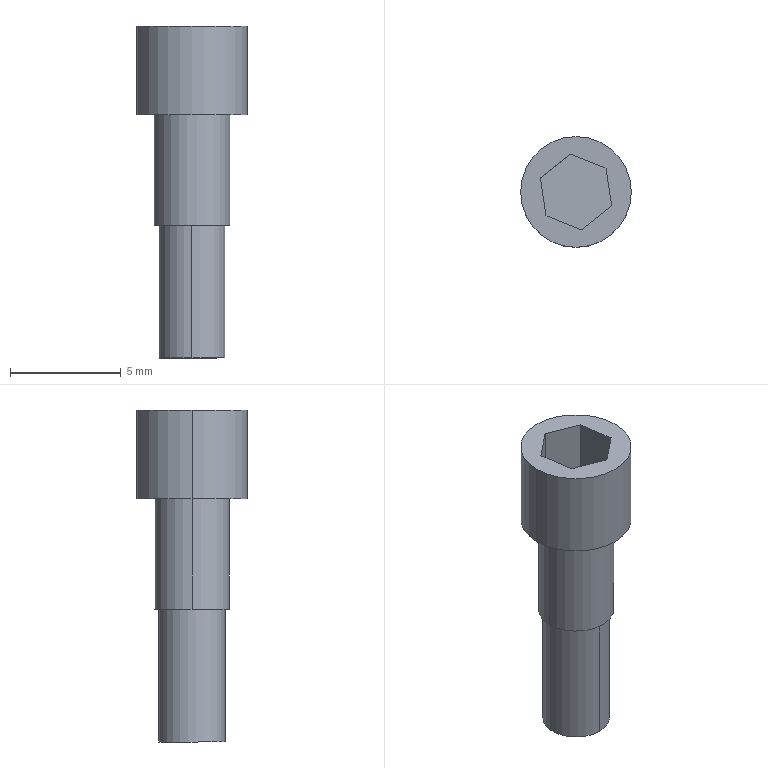Part | SolidWorks | features ICE 2, Cut 1, Extrusion 1 | 1 solid | 17 faces | box 5 x 5 x 15 mm | volume 142.965 mm3 | plane 11 | cylinder 6 | commonest cylinder face diameters 3 x2 3.4 x2 5 x2
STEP:
#1=CARTESIAN_POINT('',(2.5,-6.,4.));
#2=VERTEX_POINT('',#1);
#3=CARTESIAN_POINT('',(-2.5,-6.,4.));
#4=VERTEX_POINT('',#3);
#5=CARTESIAN_POINT('',(0.,-6.,4.));
#6=DIRECTION('',(0.,0.,1.));
#7=DIRECTION('',(1.,0.,0.));
#8=AXIS2_PLACEMENT_3D('',#5,#6,#7);
#9=CIRCLE('',#8,2.5);
#10=EDGE_CURVE('',#2,#4,#9,.T.);
#11=ORIENTED_EDGE('',*,*,#10,.F.);
#12=CARTESIAN_POINT('',(2.5,-6.,0.));
#13=VERTEX_POINT('',#12);
#14=CARTESIAN_POINT('',(2.5,-6.,4.));
#15=DIRECTION('',(0.,0.,-1.));
#16=VECTOR('',#15,1000.);
#17=LINE('',#14,#16);
#18=EDGE_CURVE('',#2,#13,#17,.T.);
#19=ORIENTED_EDGE('',*,*,#18,.T.);
#20=CARTESIAN_POINT('',(-2.5,-6.,0.));
#21=VERTEX_POINT('',#20);
#22=CARTESIAN_POINT('',(0.,-6.,0.));
#23=DIRECTION('',(0.,0.,1.));
#24=DIRECTION('',(1.,0.,0.));
#25=AXIS2_PLACEMENT_3D('',#22,#23,#24);
#26=CIRCLE('',#25,2.5);
#27=EDGE_CURVE('',#13,#21,#26,.T.);
#28=ORIENTED_EDGE('',*,*,#27,.T.);
#29=CARTESIAN_POINT('',(-2.5,-6.,4.));
#30=DIRECTION('',(0.,0.,-1.));
#31=VECTOR('',#30,1000.);
#32=LINE('',#29,#31);
#33=EDGE_CURVE('',#4,#21,#32,.T.);
#34=ORIENTED_EDGE('',*,*,#33,.F.);
#35=EDGE_LOOP('',(#11,#19,#28,#34));
#36=FACE_OUTER_BOUND('',#35,.T.);
#37=CARTESIAN_POINT('',(0.,-6.,4.));
#38=DIRECTION('',(0.,0.,-1.));
#39=DIRECTION('',(-1.,0.,0.));
#40=AXIS2_PLACEMENT_3D('',#37,#38,#39);
#41=CYLINDRICAL_SURFACE('',#40,2.5);
#42=ADVANCED_FACE('',(#36),#41,.T.);
#43=CARTESIAN_POINT('',(0.,-4.5,-11.));
#44=VERTEX_POINT('',#43);
#45=CARTESIAN_POINT('',(0.,-7.5,-11.));
#46=VERTEX_POINT('',#45);
#47=CARTESIAN_POINT('',(0.,-6.,-11.));
#48=DIRECTION('',(0.,0.,-1.));
#49=DIRECTION('',(0.,1.,0.));
#50=AXIS2_PLACEMENT_3D('',#47,#48,#49);
#51=CIRCLE('',#50,1.5);
#52=EDGE_CURVE('',#44,#46,#51,.T.);
#53=ORIENTED_EDGE('',*,*,#52,.F.);
#54=CARTESIAN_POINT('',(0.,-4.5,-5.));
#55=VERTEX_POINT('',#54);
#56=CARTESIAN_POINT('',(0.,-4.5,-11.));
#57=DIRECTION('',(0.,0.,1.));
#58=VECTOR('',#57,1000.);
#59=LINE('',#56,#58);
#60=EDGE_CURVE('',#44,#55,#59,.T.);
#61=ORIENTED_EDGE('',*,*,#60,.T.);
#62=CARTESIAN_POINT('',(0.,-7.5,-5.));
#63=VERTEX_POINT('',#62);
#64=CARTESIAN_POINT('',(0.,-6.,-5.));
#65=DIRECTION('',(0.,0.,-1.));
#66=DIRECTION('',(1.,0.,0.));
#67=AXIS2_PLACEMENT_3D('',#64,#65,#66);
#68=CIRCLE('',#67,1.5);
#69=EDGE_CURVE('',#55,#63,#68,.T.);
#70=ORIENTED_EDGE('',*,*,#69,.T.);
#71=CARTESIAN_POINT('',(0.,-7.5,-11.));
#72=DIRECTION('',(0.,0.,1.));
#73=VECTOR('',#72,1000.);
#74=LINE('',#71,#73);
#75=EDGE_CURVE('',#46,#63,#74,.T.);
#76=ORIENTED_EDGE('',*,*,#75,.F.);
#77=EDGE_LOOP('',(#53,#61,#70,#76));
#78=FACE_OUTER_BOUND('',#77,.T.);
#79=CARTESIAN_POINT('',(0.,-6.,-11.));
#80=DIRECTION('',(0.,0.,1.));
#81=DIRECTION('',(0.,-1.,0.));
#82=AXIS2_PLACEMENT_3D('',#79,#80,#81);
#83=CYLINDRICAL_SURFACE('',#82,1.5);
#84=ADVANCED_FACE('',(#78),#83,.T.);
#85=CARTESIAN_POINT('',(1.7,-6.,-5.));
#86=VERTEX_POINT('',#85);
#87=CARTESIAN_POINT('',(-1.7,-6.,-5.));
#88=VERTEX_POINT('',#87);
#89=CARTESIAN_POINT('',(0.,-6.,-5.));
#90=DIRECTION('',(0.,0.,1.));
#91=DIRECTION('',(1.,0.,0.));
#92=AXIS2_PLACEMENT_3D('',#89,#90,#91);
#93=CIRCLE('',#92,1.7);
#94=EDGE_CURVE('',#86,#88,#93,.T.);
#95=ORIENTED_EDGE('',*,*,#94,.T.);
#96=CARTESIAN_POINT('',(-1.7,-6.,0.));
#97=VERTEX_POINT('',#96);
#98=CARTESIAN_POINT('',(-1.7,-6.,-5.));
#99=DIRECTION('',(0.,0.,1.));
#100=VECTOR('',#99,1000.);
#101=LINE('',#98,#100);
#102=EDGE_CURVE('',#88,#97,#101,.T.);
#103=ORIENTED_EDGE('',*,*,#102,.T.);
#104=CARTESIAN_POINT('',(1.7,-6.,0.));
#105=VERTEX_POINT('',#104);
#106=CARTESIAN_POINT('',(0.,-6.,0.));
#107=DIRECTION('',(0.,0.,1.));
#108=DIRECTION('',(1.,0.,0.));
#109=AXIS2_PLACEMENT_3D('',#106,#107,#108);
#110=CIRCLE('',#109,1.7);
#111=EDGE_CURVE('',#105,#97,#110,.T.);
#112=ORIENTED_EDGE('',*,*,#111,.F.);
#113=CARTESIAN_POINT('',(1.7,-6.,-5.));
#114=DIRECTION('',(0.,0.,1.));
#115=VECTOR('',#114,1000.);
#116=LINE('',#113,#115);
#117=EDGE_CURVE('',#86,#105,#116,.T.);
#118=ORIENTED_EDGE('',*,*,#117,.F.);
#119=EDGE_LOOP('',(#95,#103,#112,#118));
#120=FACE_OUTER_BOUND('',#119,.T.);
#121=CARTESIAN_POINT('',(0.,-6.,-5.));
#122=DIRECTION('',(0.,0.,1.));
#123=DIRECTION('',(1.,0.,0.));
#124=AXIS2_PLACEMENT_3D('',#121,#122,#123);
#125=CYLINDRICAL_SURFACE('',#124,1.7);
#126=ADVANCED_FACE('',(#120),#125,.T.);
#127=ORIENTED_EDGE('',*,*,#102,.F.);
#128=CARTESIAN_POINT('',(0.,-6.,-5.));
#129=DIRECTION('',(0.,0.,1.));
#130=DIRECTION('',(1.,0.,0.));
#131=AXIS2_PLACEMENT_3D('',#128,#129,#130);
#132=CIRCLE('',#131,1.7);
#133=EDGE_CURVE('',#88,#86,#132,.T.);
#134=ORIENTED_EDGE('',*,*,#133,.T.);
#135=ORIENTED_EDGE('',*,*,#117,.T.);
#136=CARTESIAN_POINT('',(0.,-6.,0.));
#137=DIRECTION('',(0.,0.,1.));
#138=DIRECTION('',(1.,0.,0.));
#139=AXIS2_PLACEMENT_3D('',#136,#137,#138);
#140=CIRCLE('',#139,1.7);
#141=EDGE_CURVE('',#97,#105,#140,.T.);
#142=ORIENTED_EDGE('',*,*,#141,.F.);
#143=EDGE_LOOP('',(#127,#134,#135,#142));
#144=FACE_OUTER_BOUND('',#143,.T.);
#145=CARTESIAN_POINT('',(0.,-6.,-5.));
#146=DIRECTION('',(0.,0.,1.));
#147=DIRECTION('',(1.,0.,0.));
#148=AXIS2_PLACEMENT_3D('',#145,#146,#147);
#149=CYLINDRICAL_SURFACE('',#148,1.7);
#150=ADVANCED_FACE('',(#144),#149,.T.);
#151=CARTESIAN_POINT('',(0.,-6.,-5.));
#152=DIRECTION('',(0.,0.,-1.));
#153=DIRECTION('',(1.,0.,0.));
#154=AXIS2_PLACEMENT_3D('',#151,#152,#153);
#155=CIRCLE('',#154,1.5);
#156=EDGE_CURVE('',#63,#55,#155,.T.);
#157=ORIENTED_EDGE('',*,*,#156,.F.);
#158=ORIENTED_EDGE('',*,*,#69,.F.);
#159=EDGE_LOOP('',(#157,#158));
#160=FACE_BOUND('',#159,.T.);
#161=ORIENTED_EDGE('',*,*,#94,.F.);
#162=ORIENTED_EDGE('',*,*,#133,.F.);
#163=EDGE_LOOP('',(#161,#162));
#164=FACE_OUTER_BOUND('',#163,.T.);
#165=CARTESIAN_POINT('',(0.,-6.,-5.));
#166=DIRECTION('',(0.,0.,1.));
#167=DIRECTION('',(1.,0.,0.));
#168=AXIS2_PLACEMENT_3D('',#165,#166,#167);
#169=PLANE('',#168);
#170=ADVANCED_FACE('',(#160,#164),#169,.F.);
#171=ORIENTED_EDGE('',*,*,#60,.F.);
#172=CARTESIAN_POINT('',(0.,-6.,-11.));
#173=DIRECTION('',(0.,0.,-1.));
#174=DIRECTION('',(0.,1.,0.));
#175=AXIS2_PLACEMENT_3D('',#172,#173,#174);
#176=CIRCLE('',#175,1.5);
#177=EDGE_CURVE('',#46,#44,#176,.T.);
#178=ORIENTED_EDGE('',*,*,#177,.F.);
#179=ORIENTED_EDGE('',*,*,#75,.T.);
#180=ORIENTED_EDGE('',*,*,#156,.T.);
#181=EDGE_LOOP('',(#171,#178,#179,#180));
#182=FACE_OUTER_BOUND('',#181,.T.);
#183=CARTESIAN_POINT('',(0.,-6.,-11.));
#184=DIRECTION('',(0.,0.,1.));
#185=DIRECTION('',(0.,-1.,0.));
#186=AXIS2_PLACEMENT_3D('',#183,#184,#185);
#187=CYLINDRICAL_SURFACE('',#186,1.5);
#188=ADVANCED_FACE('',(#182),#187,.T.);
#189=ORIENTED_EDGE('',*,*,#177,.T.);
#190=ORIENTED_EDGE('',*,*,#52,.T.);
#191=EDGE_LOOP('',(#189,#190));
#192=FACE_OUTER_BOUND('',#191,.T.);
#193=CARTESIAN_POINT('',(0.,-6.,-11.));
#194=DIRECTION('',(0.,0.,-1.));
#195=DIRECTION('',(0.,1.,0.));
#196=AXIS2_PLACEMENT_3D('',#193,#194,#195);
#197=PLANE('',#196);
#198=ADVANCED_FACE('',(#192),#197,.T.);
#199=ORIENTED_EDGE('',*,*,#18,.F.);
#200=CARTESIAN_POINT('',(0.,-6.,4.));
#201=DIRECTION('',(0.,0.,1.));
#202=DIRECTION('',(1.,0.,0.));
#203=AXIS2_PLACEMENT_3D('',#200,#201,#202);
#204=CIRCLE('',#203,2.5);
#205=EDGE_CURVE('',#4,#2,#204,.T.);
#206=ORIENTED_EDGE('',*,*,#205,.F.);
#207=ORIENTED_EDGE('',*,*,#33,.T.);
#208=CARTESIAN_POINT('',(0.,-6.,0.));
#209=DIRECTION('',(0.,0.,1.));
#210=DIRECTION('',(1.,0.,0.));
#211=AXIS2_PLACEMENT_3D('',#208,#209,#210);
#212=CIRCLE('',#211,2.5);
#213=EDGE_CURVE('',#21,#13,#212,.T.);
#214=ORIENTED_EDGE('',*,*,#213,.T.);
#215=EDGE_LOOP('',(#199,#206,#207,#214));
#216=FACE_OUTER_BOUND('',#215,.T.);
#217=CARTESIAN_POINT('',(0.,-6.,4.));
#218=DIRECTION('',(0.,0.,-1.));
#219=DIRECTION('',(-1.,0.,0.));
#220=AXIS2_PLACEMENT_3D('',#217,#218,#219);
#221=CYLINDRICAL_SURFACE('',#220,2.5);
#222=ADVANCED_FACE('',(#216),#221,.T.);
#223=CARTESIAN_POINT('',(1.612,-6.635,4.));
#224=VERTEX_POINT('',#223);
#225=CARTESIAN_POINT('',(1.356,-4.922,4.));
#226=VERTEX_POINT('',#225);
#227=CARTESIAN_POINT('',(1.612,-6.635,4.));
#228=DIRECTION('',(-0.1478,0.989,0.));
#229=VECTOR('',#228,1000.);
#230=LINE('',#227,#229);
#231=EDGE_CURVE('',#224,#226,#230,.T.);
#232=ORIENTED_EDGE('',*,*,#231,.F.);
#233=CARTESIAN_POINT('',(0.256,-7.713,4.));
#234=VERTEX_POINT('',#233);
#235=CARTESIAN_POINT('',(0.256,-7.713,4.));
#236=DIRECTION('',(0.7826,0.6225,0.));
#237=VECTOR('',#236,1000.);
#238=LINE('',#235,#237);
#239=EDGE_CURVE('',#234,#224,#238,.T.);
#240=ORIENTED_EDGE('',*,*,#239,.F.);
#241=CARTESIAN_POINT('',(-1.356,-7.078,4.));
#242=VERTEX_POINT('',#241);
#243=CARTESIAN_POINT('',(-1.356,-7.078,4.));
#244=DIRECTION('',(0.9304,-0.3665,0.));
#245=VECTOR('',#244,1000.);
#246=LINE('',#243,#245);
#247=EDGE_CURVE('',#242,#234,#246,.T.);
#248=ORIENTED_EDGE('',*,*,#247,.F.);
#249=CARTESIAN_POINT('',(-1.612,-5.365,4.));
#250=VERTEX_POINT('',#249);
#251=CARTESIAN_POINT('',(-1.612,-5.365,4.));
#252=DIRECTION('',(0.1478,-0.989,0.));
#253=VECTOR('',#252,1000.);
#254=LINE('',#251,#253);
#255=EDGE_CURVE('',#250,#242,#254,.T.);
#256=ORIENTED_EDGE('',*,*,#255,.F.);
#257=CARTESIAN_POINT('',(-0.256,-4.287,4.));
#258=VERTEX_POINT('',#257);
#259=CARTESIAN_POINT('',(-0.256,-4.287,4.));
#260=DIRECTION('',(-0.7826,-0.6225,0.));
#261=VECTOR('',#260,1000.);
#262=LINE('',#259,#261);
#263=EDGE_CURVE('',#258,#250,#262,.T.);
#264=ORIENTED_EDGE('',*,*,#263,.F.);
#265=CARTESIAN_POINT('',(1.356,-4.922,4.));
#266=DIRECTION('',(-0.9304,0.3665,0.));
#267=VECTOR('',#266,1000.);
#268=LINE('',#265,#267);
#269=EDGE_CURVE('',#226,#258,#268,.T.);
#270=ORIENTED_EDGE('',*,*,#269,.F.);
#271=EDGE_LOOP('',(#232,#240,#248,#256,#264,#270));
#272=FACE_BOUND('',#271,.T.);
#273=ORIENTED_EDGE('',*,*,#205,.T.);
#274=ORIENTED_EDGE('',*,*,#10,.T.);
#275=EDGE_LOOP('',(#273,#274));
#276=FACE_OUTER_BOUND('',#275,.T.);
#277=CARTESIAN_POINT('',(0.,-6.,4.));
#278=DIRECTION('',(0.,0.,1.));
#279=DIRECTION('',(1.,0.,0.));
#280=AXIS2_PLACEMENT_3D('',#277,#278,#279);
#281=PLANE('',#280);
#282=ADVANCED_FACE('',(#272,#276),#281,.T.);
#283=ORIENTED_EDGE('',*,*,#111,.T.);
#284=ORIENTED_EDGE('',*,*,#141,.T.);
#285=EDGE_LOOP('',(#283,#284));
#286=FACE_BOUND('',#285,.T.);
#287=ORIENTED_EDGE('',*,*,#213,.F.);
#288=ORIENTED_EDGE('',*,*,#27,.F.);
#289=EDGE_LOOP('',(#287,#288));
#290=FACE_OUTER_BOUND('',#289,.T.);
#291=CARTESIAN_POINT('',(0.,-6.,0.));
#292=DIRECTION('',(0.,0.,1.));
#293=DIRECTION('',(1.,0.,0.));
#294=AXIS2_PLACEMENT_3D('',#291,#292,#293);
#295=PLANE('',#294);
#296=ADVANCED_FACE('',(#286,#290),#295,.F.);
#297=ORIENTED_EDGE('',*,*,#231,.T.);
#298=CARTESIAN_POINT('',(1.356,-4.922,1.));
#299=VERTEX_POINT('',#298);
#300=CARTESIAN_POINT('',(1.356,-4.922,1.));
#301=DIRECTION('',(0.,0.,1.));
#302=VECTOR('',#301,1000.);
#303=LINE('',#300,#302);
#304=EDGE_CURVE('',#299,#226,#303,.T.);
#305=ORIENTED_EDGE('',*,*,#304,.F.);
#306=CARTESIAN_POINT('',(1.612,-6.635,1.));
#307=VERTEX_POINT('',#306);
#308=CARTESIAN_POINT('',(1.612,-6.635,1.));
#309=DIRECTION('',(-0.1478,0.989,0.));
#310=VECTOR('',#309,1000.);
#311=LINE('',#308,#310);
#312=EDGE_CURVE('',#307,#299,#311,.T.);
#313=ORIENTED_EDGE('',*,*,#312,.F.);
#314=CARTESIAN_POINT('',(1.612,-6.635,1.));
#315=DIRECTION('',(0.,0.,1.));
#316=VECTOR('',#315,1000.);
#317=LINE('',#314,#316);
#318=EDGE_CURVE('',#307,#224,#317,.T.);
#319=ORIENTED_EDGE('',*,*,#318,.T.);
#320=EDGE_LOOP('',(#297,#305,#313,#319));
#321=FACE_OUTER_BOUND('',#320,.T.);
#322=CARTESIAN_POINT('',(1.612,-6.635,1.));
#323=DIRECTION('',(0.989,0.1478,0.));
#324=DIRECTION('',(-0.1478,0.989,0.));
#325=AXIS2_PLACEMENT_3D('',#322,#323,#324);
#326=PLANE('',#325);
#327=ADVANCED_FACE('',(#321),#326,.F.);
#328=ORIENTED_EDGE('',*,*,#239,.T.);
#329=ORIENTED_EDGE('',*,*,#318,.F.);
#330=CARTESIAN_POINT('',(0.256,-7.713,1.));
#331=VERTEX_POINT('',#330);
#332=CARTESIAN_POINT('',(0.256,-7.713,1.));
#333=DIRECTION('',(0.7826,0.6225,0.));
#334=VECTOR('',#333,1000.);
#335=LINE('',#332,#334);
#336=EDGE_CURVE('',#331,#307,#335,.T.);
#337=ORIENTED_EDGE('',*,*,#336,.F.);
#338=CARTESIAN_POINT('',(0.256,-7.713,1.));
#339=DIRECTION('',(0.,0.,1.));
#340=VECTOR('',#339,1000.);
#341=LINE('',#338,#340);
#342=EDGE_CURVE('',#331,#234,#341,.T.);
#343=ORIENTED_EDGE('',*,*,#342,.T.);
#344=EDGE_LOOP('',(#328,#329,#337,#343));
#345=FACE_OUTER_BOUND('',#344,.T.);
#346=CARTESIAN_POINT('',(0.256,-7.713,1.));
#347=DIRECTION('',(0.6225,-0.7826,0.));
#348=DIRECTION('',(0.7826,0.6225,0.));
#349=AXIS2_PLACEMENT_3D('',#346,#347,#348);
#350=PLANE('',#349);
#351=ADVANCED_FACE('',(#345),#350,.F.);
#352=ORIENTED_EDGE('',*,*,#247,.T.);
#353=ORIENTED_EDGE('',*,*,#342,.F.);
#354=CARTESIAN_POINT('',(-1.356,-7.078,1.));
#355=VERTEX_POINT('',#354);
#356=CARTESIAN_POINT('',(-1.356,-7.078,1.));
#357=DIRECTION('',(0.9304,-0.3665,0.));
#358=VECTOR('',#357,1000.);
#359=LINE('',#356,#358);
#360=EDGE_CURVE('',#355,#331,#359,.T.);
#361=ORIENTED_EDGE('',*,*,#360,.F.);
#362=CARTESIAN_POINT('',(-1.356,-7.078,1.));
#363=DIRECTION('',(0.,0.,1.));
#364=VECTOR('',#363,1000.);
#365=LINE('',#362,#364);
#366=EDGE_CURVE('',#355,#242,#365,.T.);
#367=ORIENTED_EDGE('',*,*,#366,.T.);
#368=EDGE_LOOP('',(#352,#353,#361,#367));
#369=FACE_OUTER_BOUND('',#368,.T.);
#370=CARTESIAN_POINT('',(-1.356,-7.078,1.));
#371=DIRECTION('',(-0.3665,-0.9304,0.));
#372=DIRECTION('',(0.9304,-0.3665,0.));
#373=AXIS2_PLACEMENT_3D('',#370,#371,#372);
#374=PLANE('',#373);
#375=ADVANCED_FACE('',(#369),#374,.F.);
#376=ORIENTED_EDGE('',*,*,#255,.T.);
#377=ORIENTED_EDGE('',*,*,#366,.F.);
#378=CARTESIAN_POINT('',(-1.612,-5.365,1.));
#379=VERTEX_POINT('',#378);
#380=CARTESIAN_POINT('',(-1.612,-5.365,1.));
#381=DIRECTION('',(0.1478,-0.989,0.));
#382=VECTOR('',#381,1000.);
#383=LINE('',#380,#382);
#384=EDGE_CURVE('',#379,#355,#383,.T.);
#385=ORIENTED_EDGE('',*,*,#384,.F.);
#386=CARTESIAN_POINT('',(-1.612,-5.365,1.));
#387=DIRECTION('',(0.,0.,1.));
#388=VECTOR('',#387,1000.);
#389=LINE('',#386,#388);
#390=EDGE_CURVE('',#379,#250,#389,.T.);
#391=ORIENTED_EDGE('',*,*,#390,.T.);
#392=EDGE_LOOP('',(#376,#377,#385,#391));
#393=FACE_OUTER_BOUND('',#392,.T.);
#394=CARTESIAN_POINT('',(-1.612,-5.365,1.));
#395=DIRECTION('',(-0.989,-0.1478,0.));
#396=DIRECTION('',(0.1478,-0.989,0.));
#397=AXIS2_PLACEMENT_3D('',#394,#395,#396);
#398=PLANE('',#397);
#399=ADVANCED_FACE('',(#393),#398,.F.);
#400=ORIENTED_EDGE('',*,*,#263,.T.);
#401=ORIENTED_EDGE('',*,*,#390,.F.);
#402=CARTESIAN_POINT('',(-0.256,-4.287,1.));
#403=VERTEX_POINT('',#402);
#404=CARTESIAN_POINT('',(-0.256,-4.287,1.));
#405=DIRECTION('',(-0.7826,-0.6225,0.));
#406=VECTOR('',#405,1000.);
#407=LINE('',#404,#406);
#408=EDGE_CURVE('',#403,#379,#407,.T.);
#409=ORIENTED_EDGE('',*,*,#408,.F.);
#410=CARTESIAN_POINT('',(-0.256,-4.287,1.));
#411=DIRECTION('',(0.,0.,1.));
#412=VECTOR('',#411,1000.);
#413=LINE('',#410,#412);
#414=EDGE_CURVE('',#403,#258,#413,.T.);
#415=ORIENTED_EDGE('',*,*,#414,.T.);
#416=EDGE_LOOP('',(#400,#401,#409,#415));
#417=FACE_OUTER_BOUND('',#416,.T.);
#418=CARTESIAN_POINT('',(-0.256,-4.287,1.));
#419=DIRECTION('',(-0.6225,0.7826,0.));
#420=DIRECTION('',(-0.7826,-0.6225,0.));
#421=AXIS2_PLACEMENT_3D('',#418,#419,#420);
#422=PLANE('',#421);
#423=ADVANCED_FACE('',(#417),#422,.F.);
#424=ORIENTED_EDGE('',*,*,#269,.T.);
#425=ORIENTED_EDGE('',*,*,#414,.F.);
#426=CARTESIAN_POINT('',(1.356,-4.922,1.));
#427=DIRECTION('',(-0.9304,0.3665,0.));
#428=VECTOR('',#427,1000.);
#429=LINE('',#426,#428);
#430=EDGE_CURVE('',#299,#403,#429,.T.);
#431=ORIENTED_EDGE('',*,*,#430,.F.);
#432=ORIENTED_EDGE('',*,*,#304,.T.);
#433=EDGE_LOOP('',(#424,#425,#431,#432));
#434=FACE_OUTER_BOUND('',#433,.T.);
#435=CARTESIAN_POINT('',(1.356,-4.922,1.));
#436=DIRECTION('',(0.3665,0.9304,0.));
#437=DIRECTION('',(-0.9304,0.3665,0.));
#438=AXIS2_PLACEMENT_3D('',#435,#436,#437);
#439=PLANE('',#438);
#440=ADVANCED_FACE('',(#434),#439,.F.);
#441=ORIENTED_EDGE('',*,*,#312,.T.);
#442=ORIENTED_EDGE('',*,*,#430,.T.);
#443=ORIENTED_EDGE('',*,*,#408,.T.);
#444=ORIENTED_EDGE('',*,*,#384,.T.);
#445=ORIENTED_EDGE('',*,*,#360,.T.);
#446=ORIENTED_EDGE('',*,*,#336,.T.);
#447=EDGE_LOOP('',(#441,#442,#443,#444,#445,#446));
#448=FACE_OUTER_BOUND('',#447,.T.);
#449=CARTESIAN_POINT('',(0.,0.,1.));
#450=DIRECTION('',(0.,0.,1.));
#451=DIRECTION('',(1.,0.,0.));
#452=AXIS2_PLACEMENT_3D('',#449,#450,#451);
#453=PLANE('',#452);
#454=ADVANCED_FACE('',(#448),#453,.T.);
#455=CLOSED_SHELL('',(#42,#84,#126,#150,#170,#188,#198,#222,#282,#296,#327,#351,#375,#399,#423,#440,#454));
#456=MANIFOLD_SOLID_BREP('',#455);
#457=CARTESIAN_POINT('',(0.,0.,0.));
#458=DIRECTION('',(0.,0.,1.));
#459=DIRECTION('',(1.,0.,0.));
#460=AXIS2_PLACEMENT_3D('',#457,#458,#459);
#461=(LENGTH_UNIT()NAMED_UNIT(*)SI_UNIT(.MILLI.,.METRE.));
#462=UNCERTAINTY_MEASURE_WITH_UNIT(LENGTH_MEASURE(0.00001),#461,'','');
#463=(NAMED_UNIT(*)PLANE_ANGLE_UNIT()SI_UNIT($,.RADIAN.));
#464=(NAMED_UNIT(*)SI_UNIT($,.STERADIAN.)SOLID_ANGLE_UNIT());
#465=(GEOMETRIC_REPRESENTATION_CONTEXT(3)GLOBAL_UNCERTAINTY_ASSIGNED_CONTEXT((#462))GLOBAL_UNIT_ASSIGNED_CONTEXT((#461,#463,#464))REPRESENTATION_CONTEXT('',''));
#466=ADVANCED_BREP_SHAPE_REPRESENTATION('',(#456,#460),#465);